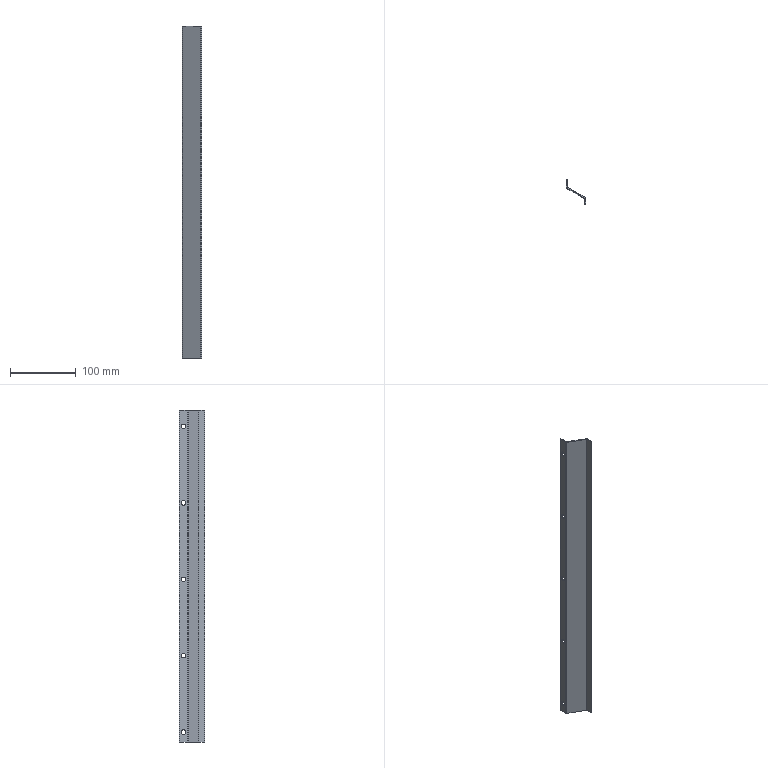Part | STEP file | Right Small Door Splash Plate | 1 solid | 24 faces | box 29.5 x 38.166 x 504 mm | volume 40648 mm3 | cylinder 14 | plane 10 | commonest cylinder face diameters 7 x10 0.2 x2 3.2 x2
STEP:
#1=CARTESIAN_POINT('',(-46.603,-10.206,479.));
#2=VERTEX_POINT('',#1);
#3=CARTESIAN_POINT('',(-46.603,-3.206,479.));
#4=VERTEX_POINT('',#3);
#5=CARTESIAN_POINT('',(-46.603,-6.706,479.));
#6=DIRECTION('',(1.,0.,0.));
#7=DIRECTION('',(0.,1.,0.));
#8=AXIS2_PLACEMENT_3D('',#5,#6,#7);
#9=CIRCLE('',#8,3.5);
#10=EDGE_CURVE('',#2,#4,#9,.T.);
#11=ORIENTED_EDGE('',*,*,#10,.F.);
#12=CARTESIAN_POINT('',(-45.103,-10.206,479.));
#13=VERTEX_POINT('',#12);
#14=CARTESIAN_POINT('',(-55.103,-10.206,479.));
#15=DIRECTION('',(1.,0.,0.));
#16=VECTOR('',#15,1000.);
#17=LINE('',#14,#16);
#18=EDGE_CURVE('',#2,#13,#17,.T.);
#19=ORIENTED_EDGE('',*,*,#18,.T.);
#20=CARTESIAN_POINT('',(-45.103,-3.206,479.));
#21=VERTEX_POINT('',#20);
#22=CARTESIAN_POINT('',(-45.103,-6.706,479.));
#23=DIRECTION('',(-1.,0.,0.));
#24=DIRECTION('',(0.,1.,0.));
#25=AXIS2_PLACEMENT_3D('',#22,#23,#24);
#26=CIRCLE('',#25,3.5);
#27=EDGE_CURVE('',#21,#13,#26,.T.);
#28=ORIENTED_EDGE('',*,*,#27,.F.);
#29=CARTESIAN_POINT('',(-55.103,-3.206,479.));
#30=DIRECTION('',(1.,0.,0.));
#31=VECTOR('',#30,1000.);
#32=LINE('',#29,#31);
#33=EDGE_CURVE('',#4,#21,#32,.T.);
#34=ORIENTED_EDGE('',*,*,#33,.F.);
#35=EDGE_LOOP('',(#11,#19,#28,#34));
#36=FACE_OUTER_BOUND('',#35,.T.);
#37=CARTESIAN_POINT('',(-55.103,-6.706,479.));
#38=DIRECTION('',(1.,0.,0.));
#39=DIRECTION('',(0.,1.,0.));
#40=AXIS2_PLACEMENT_3D('',#37,#38,#39);
#41=CYLINDRICAL_SURFACE('',#40,3.5);
#42=ADVANCED_FACE('',(#36),#41,.F.);
#43=CARTESIAN_POINT('',(-46.603,-10.206,363.));
#44=VERTEX_POINT('',#43);
#45=CARTESIAN_POINT('',(-46.603,-3.206,363.));
#46=VERTEX_POINT('',#45);
#47=CARTESIAN_POINT('',(-46.603,-6.706,363.));
#48=DIRECTION('',(1.,0.,0.));
#49=DIRECTION('',(0.,1.,0.));
#50=AXIS2_PLACEMENT_3D('',#47,#48,#49);
#51=CIRCLE('',#50,3.5);
#52=EDGE_CURVE('',#44,#46,#51,.T.);
#53=ORIENTED_EDGE('',*,*,#52,.F.);
#54=CARTESIAN_POINT('',(-45.103,-10.206,363.));
#55=VERTEX_POINT('',#54);
#56=CARTESIAN_POINT('',(-55.103,-10.206,363.));
#57=DIRECTION('',(1.,0.,0.));
#58=VECTOR('',#57,1000.);
#59=LINE('',#56,#58);
#60=EDGE_CURVE('',#44,#55,#59,.T.);
#61=ORIENTED_EDGE('',*,*,#60,.T.);
#62=CARTESIAN_POINT('',(-45.103,-3.206,363.));
#63=VERTEX_POINT('',#62);
#64=CARTESIAN_POINT('',(-45.103,-6.706,363.));
#65=DIRECTION('',(-1.,0.,0.));
#66=DIRECTION('',(0.,1.,0.));
#67=AXIS2_PLACEMENT_3D('',#64,#65,#66);
#68=CIRCLE('',#67,3.5);
#69=EDGE_CURVE('',#63,#55,#68,.T.);
#70=ORIENTED_EDGE('',*,*,#69,.F.);
#71=CARTESIAN_POINT('',(-55.103,-3.206,363.));
#72=DIRECTION('',(1.,0.,0.));
#73=VECTOR('',#72,1000.);
#74=LINE('',#71,#73);
#75=EDGE_CURVE('',#46,#63,#74,.T.);
#76=ORIENTED_EDGE('',*,*,#75,.F.);
#77=EDGE_LOOP('',(#53,#61,#70,#76));
#78=FACE_OUTER_BOUND('',#77,.T.);
#79=CARTESIAN_POINT('',(-55.103,-6.706,363.));
#80=DIRECTION('',(1.,0.,0.));
#81=DIRECTION('',(0.,1.,0.));
#82=AXIS2_PLACEMENT_3D('',#79,#80,#81);
#83=CYLINDRICAL_SURFACE('',#82,3.5);
#84=ADVANCED_FACE('',(#78),#83,.F.);
#85=CARTESIAN_POINT('',(-46.603,-10.206,247.));
#86=VERTEX_POINT('',#85);
#87=CARTESIAN_POINT('',(-46.603,-3.206,247.));
#88=VERTEX_POINT('',#87);
#89=CARTESIAN_POINT('',(-46.603,-6.706,247.));
#90=DIRECTION('',(1.,0.,0.));
#91=DIRECTION('',(0.,1.,0.));
#92=AXIS2_PLACEMENT_3D('',#89,#90,#91);
#93=CIRCLE('',#92,3.5);
#94=EDGE_CURVE('',#86,#88,#93,.T.);
#95=ORIENTED_EDGE('',*,*,#94,.F.);
#96=CARTESIAN_POINT('',(-45.103,-10.206,247.));
#97=VERTEX_POINT('',#96);
#98=CARTESIAN_POINT('',(-55.103,-10.206,247.));
#99=DIRECTION('',(1.,0.,0.));
#100=VECTOR('',#99,1000.);
#101=LINE('',#98,#100);
#102=EDGE_CURVE('',#86,#97,#101,.T.);
#103=ORIENTED_EDGE('',*,*,#102,.T.);
#104=CARTESIAN_POINT('',(-45.103,-3.206,247.));
#105=VERTEX_POINT('',#104);
#106=CARTESIAN_POINT('',(-45.103,-6.706,247.));
#107=DIRECTION('',(-1.,0.,0.));
#108=DIRECTION('',(0.,1.,0.));
#109=AXIS2_PLACEMENT_3D('',#106,#107,#108);
#110=CIRCLE('',#109,3.5);
#111=EDGE_CURVE('',#105,#97,#110,.T.);
#112=ORIENTED_EDGE('',*,*,#111,.F.);
#113=CARTESIAN_POINT('',(-55.103,-3.206,247.));
#114=DIRECTION('',(1.,0.,0.));
#115=VECTOR('',#114,1000.);
#116=LINE('',#113,#115);
#117=EDGE_CURVE('',#88,#105,#116,.T.);
#118=ORIENTED_EDGE('',*,*,#117,.F.);
#119=EDGE_LOOP('',(#95,#103,#112,#118));
#120=FACE_OUTER_BOUND('',#119,.T.);
#121=CARTESIAN_POINT('',(-55.103,-6.706,247.));
#122=DIRECTION('',(1.,0.,0.));
#123=DIRECTION('',(0.,1.,0.));
#124=AXIS2_PLACEMENT_3D('',#121,#122,#123);
#125=CYLINDRICAL_SURFACE('',#124,3.5);
#126=ADVANCED_FACE('',(#120),#125,.F.);
#127=CARTESIAN_POINT('',(-46.603,-10.206,131.));
#128=VERTEX_POINT('',#127);
#129=CARTESIAN_POINT('',(-46.603,-3.206,131.));
#130=VERTEX_POINT('',#129);
#131=CARTESIAN_POINT('',(-46.603,-6.706,131.));
#132=DIRECTION('',(1.,0.,0.));
#133=DIRECTION('',(0.,1.,0.));
#134=AXIS2_PLACEMENT_3D('',#131,#132,#133);
#135=CIRCLE('',#134,3.5);
#136=EDGE_CURVE('',#128,#130,#135,.T.);
#137=ORIENTED_EDGE('',*,*,#136,.F.);
#138=CARTESIAN_POINT('',(-45.103,-10.206,131.));
#139=VERTEX_POINT('',#138);
#140=CARTESIAN_POINT('',(-55.103,-10.206,131.));
#141=DIRECTION('',(1.,0.,0.));
#142=VECTOR('',#141,1000.);
#143=LINE('',#140,#142);
#144=EDGE_CURVE('',#128,#139,#143,.T.);
#145=ORIENTED_EDGE('',*,*,#144,.T.);
#146=CARTESIAN_POINT('',(-45.103,-3.206,131.));
#147=VERTEX_POINT('',#146);
#148=CARTESIAN_POINT('',(-45.103,-6.706,131.));
#149=DIRECTION('',(-1.,0.,0.));
#150=DIRECTION('',(0.,1.,0.));
#151=AXIS2_PLACEMENT_3D('',#148,#149,#150);
#152=CIRCLE('',#151,3.5);
#153=EDGE_CURVE('',#147,#139,#152,.T.);
#154=ORIENTED_EDGE('',*,*,#153,.F.);
#155=CARTESIAN_POINT('',(-55.103,-3.206,131.));
#156=DIRECTION('',(1.,0.,0.));
#157=VECTOR('',#156,1000.);
#158=LINE('',#155,#157);
#159=EDGE_CURVE('',#130,#147,#158,.T.);
#160=ORIENTED_EDGE('',*,*,#159,.F.);
#161=EDGE_LOOP('',(#137,#145,#154,#160));
#162=FACE_OUTER_BOUND('',#161,.T.);
#163=CARTESIAN_POINT('',(-55.103,-6.706,131.));
#164=DIRECTION('',(1.,0.,0.));
#165=DIRECTION('',(0.,1.,0.));
#166=AXIS2_PLACEMENT_3D('',#163,#164,#165);
#167=CYLINDRICAL_SURFACE('',#166,3.5);
#168=ADVANCED_FACE('',(#162),#167,.F.);
#169=CARTESIAN_POINT('',(-46.603,-10.206,15.));
#170=VERTEX_POINT('',#169);
#171=CARTESIAN_POINT('',(-46.603,-3.206,15.));
#172=VERTEX_POINT('',#171);
#173=CARTESIAN_POINT('',(-46.603,-6.706,15.));
#174=DIRECTION('',(1.,0.,0.));
#175=DIRECTION('',(0.,1.,0.));
#176=AXIS2_PLACEMENT_3D('',#173,#174,#175);
#177=CIRCLE('',#176,3.5);
#178=EDGE_CURVE('',#170,#172,#177,.T.);
#179=ORIENTED_EDGE('',*,*,#178,.F.);
#180=CARTESIAN_POINT('',(-45.103,-10.206,15.));
#181=VERTEX_POINT('',#180);
#182=CARTESIAN_POINT('',(-55.103,-10.206,15.));
#183=DIRECTION('',(1.,0.,0.));
#184=VECTOR('',#183,1000.);
#185=LINE('',#182,#184);
#186=EDGE_CURVE('',#170,#181,#185,.T.);
#187=ORIENTED_EDGE('',*,*,#186,.T.);
#188=CARTESIAN_POINT('',(-45.103,-3.206,15.));
#189=VERTEX_POINT('',#188);
#190=CARTESIAN_POINT('',(-45.103,-6.706,15.));
#191=DIRECTION('',(-1.,0.,0.));
#192=DIRECTION('',(0.,1.,0.));
#193=AXIS2_PLACEMENT_3D('',#190,#191,#192);
#194=CIRCLE('',#193,3.5);
#195=EDGE_CURVE('',#189,#181,#194,.T.);
#196=ORIENTED_EDGE('',*,*,#195,.F.);
#197=CARTESIAN_POINT('',(-55.103,-3.206,15.));
#198=DIRECTION('',(1.,0.,0.));
#199=VECTOR('',#198,1000.);
#200=LINE('',#197,#199);
#201=EDGE_CURVE('',#172,#189,#200,.T.);
#202=ORIENTED_EDGE('',*,*,#201,.F.);
#203=EDGE_LOOP('',(#179,#187,#196,#202));
#204=FACE_OUTER_BOUND('',#203,.T.);
#205=CARTESIAN_POINT('',(-55.103,-6.706,15.));
#206=DIRECTION('',(1.,0.,0.));
#207=DIRECTION('',(0.,1.,0.));
#208=AXIS2_PLACEMENT_3D('',#205,#206,#207);
#209=CYLINDRICAL_SURFACE('',#208,3.5);
#210=ADVANCED_FACE('',(#204),#209,.F.);
#211=CARTESIAN_POINT('',(-45.053,-12.764,504.));
#212=VERTEX_POINT('',#211);
#213=CARTESIAN_POINT('',(-17.903,-28.439,504.));
#214=VERTEX_POINT('',#213);
#215=CARTESIAN_POINT('',(-45.103,-12.735,504.));
#216=DIRECTION('',(0.866,-0.5,0.));
#217=VECTOR('',#216,1000.);
#218=LINE('',#215,#217);
#219=EDGE_CURVE('',#212,#214,#218,.T.);
#220=ORIENTED_EDGE('',*,*,#219,.T.);
#221=CARTESIAN_POINT('',(-17.903,-28.439,0.));
#222=VERTEX_POINT('',#221);
#223=CARTESIAN_POINT('',(-17.903,-28.439,504.));
#224=DIRECTION('',(0.,0.,-1.));
#225=VECTOR('',#224,1000.);
#226=LINE('',#223,#225);
#227=EDGE_CURVE('',#214,#222,#226,.T.);
#228=ORIENTED_EDGE('',*,*,#227,.T.);
#229=CARTESIAN_POINT('',(-45.053,-12.764,0.));
#230=VERTEX_POINT('',#229);
#231=CARTESIAN_POINT('',(-45.103,-12.735,0.));
#232=DIRECTION('',(-0.866,0.5,0.));
#233=VECTOR('',#232,1000.);
#234=LINE('',#231,#233);
#235=EDGE_CURVE('',#222,#230,#234,.T.);
#236=ORIENTED_EDGE('',*,*,#235,.T.);
#237=CARTESIAN_POINT('',(-45.053,-12.764,504.));
#238=DIRECTION('',(0.,0.,1.));
#239=VECTOR('',#238,1000.);
#240=LINE('',#237,#239);
#241=EDGE_CURVE('',#230,#212,#240,.T.);
#242=ORIENTED_EDGE('',*,*,#241,.T.);
#243=EDGE_LOOP('',(#220,#228,#236,#242));
#244=FACE_OUTER_BOUND('',#243,.T.);
#245=CARTESIAN_POINT('',(-45.103,-12.735,504.));
#246=DIRECTION('',(0.5,0.866,0.));
#247=DIRECTION('',(-0.866,0.5,0.));
#248=AXIS2_PLACEMENT_3D('',#245,#246,#247);
#249=PLANE('',#248);
#250=ADVANCED_FACE('',(#244),#249,.T.);
#251=CARTESIAN_POINT('',(-17.103,-29.824,504.));
#252=VERTEX_POINT('',#251);
#253=CARTESIAN_POINT('',(-18.703,-29.824,504.));
#254=DIRECTION('',(0.,0.,-1.));
#255=DIRECTION('',(-1.,0.,0.));
#256=AXIS2_PLACEMENT_3D('',#253,#254,#255);
#257=CIRCLE('',#256,1.6);
#258=EDGE_CURVE('',#214,#252,#257,.T.);
#259=ORIENTED_EDGE('',*,*,#258,.T.);
#260=CARTESIAN_POINT('',(-17.103,-29.824,0.));
#261=VERTEX_POINT('',#260);
#262=CARTESIAN_POINT('',(-17.103,-29.824,504.));
#263=DIRECTION('',(0.,0.,-1.));
#264=VECTOR('',#263,1000.);
#265=LINE('',#262,#264);
#266=EDGE_CURVE('',#252,#261,#265,.T.);
#267=ORIENTED_EDGE('',*,*,#266,.T.);
#268=CARTESIAN_POINT('',(-18.703,-29.824,0.));
#269=DIRECTION('',(0.,0.,1.));
#270=DIRECTION('',(-1.,0.,0.));
#271=AXIS2_PLACEMENT_3D('',#268,#269,#270);
#272=CIRCLE('',#271,1.6);
#273=EDGE_CURVE('',#261,#222,#272,.T.);
#274=ORIENTED_EDGE('',*,*,#273,.T.);
#275=ORIENTED_EDGE('',*,*,#227,.F.);
#276=EDGE_LOOP('',(#259,#267,#274,#275));
#277=FACE_OUTER_BOUND('',#276,.T.);
#278=CARTESIAN_POINT('',(-18.703,-29.824,504.));
#279=DIRECTION('',(0.,0.,-1.));
#280=DIRECTION('',(-1.,0.,0.));
#281=AXIS2_PLACEMENT_3D('',#278,#279,#280);
#282=CYLINDRICAL_SURFACE('',#281,1.6);
#283=ADVANCED_FACE('',(#277),#282,.T.);
#284=CARTESIAN_POINT('',(-45.803,-14.063,504.));
#285=VERTEX_POINT('',#284);
#286=CARTESIAN_POINT('',(-18.653,-29.738,504.));
#287=VERTEX_POINT('',#286);
#288=CARTESIAN_POINT('',(-45.803,-14.063,504.));
#289=DIRECTION('',(0.866,-0.5,0.));
#290=VECTOR('',#289,1000.);
#291=LINE('',#288,#290);
#292=EDGE_CURVE('',#285,#287,#291,.T.);
#293=ORIENTED_EDGE('',*,*,#292,.T.);
#294=CARTESIAN_POINT('',(-18.603,-29.824,504.));
#295=VERTEX_POINT('',#294);
#296=CARTESIAN_POINT('',(-18.703,-29.824,504.));
#297=DIRECTION('',(0.,0.,-1.));
#298=DIRECTION('',(-1.,0.,0.));
#299=AXIS2_PLACEMENT_3D('',#296,#297,#298);
#300=CIRCLE('',#299,0.1);
#301=EDGE_CURVE('',#287,#295,#300,.T.);
#302=ORIENTED_EDGE('',*,*,#301,.T.);
#303=CARTESIAN_POINT('',(-18.603,-38.901,504.));
#304=VERTEX_POINT('',#303);
#305=CARTESIAN_POINT('',(-18.603,-29.738,504.));
#306=DIRECTION('',(0.,-1.,0.));
#307=VECTOR('',#306,1000.);
#308=LINE('',#305,#307);
#309=EDGE_CURVE('',#295,#304,#308,.T.);
#310=ORIENTED_EDGE('',*,*,#309,.T.);
#311=CARTESIAN_POINT('',(-17.103,-38.901,504.));
#312=VERTEX_POINT('',#311);
#313=CARTESIAN_POINT('',(-17.103,-38.901,504.));
#314=DIRECTION('',(-1.,0.,0.));
#315=VECTOR('',#314,1000.);
#316=LINE('',#313,#315);
#317=EDGE_CURVE('',#312,#304,#316,.T.);
#318=ORIENTED_EDGE('',*,*,#317,.F.);
#319=CARTESIAN_POINT('',(-17.103,-28.901,504.));
#320=DIRECTION('',(0.,-1.,0.));
#321=VECTOR('',#320,1000.);
#322=LINE('',#319,#321);
#323=EDGE_CURVE('',#252,#312,#322,.T.);
#324=ORIENTED_EDGE('',*,*,#323,.F.);
#325=ORIENTED_EDGE('',*,*,#258,.F.);
#326=ORIENTED_EDGE('',*,*,#219,.F.);
#327=CARTESIAN_POINT('',(-45.103,-12.677,504.));
#328=VERTEX_POINT('',#327);
#329=CARTESIAN_POINT('',(-45.003,-12.677,504.));
#330=DIRECTION('',(0.,0.,-1.));
#331=DIRECTION('',(-1.,0.,0.));
#332=AXIS2_PLACEMENT_3D('',#329,#330,#331);
#333=CIRCLE('',#332,0.1);
#334=EDGE_CURVE('',#212,#328,#333,.T.);
#335=ORIENTED_EDGE('',*,*,#334,.T.);
#336=CARTESIAN_POINT('',(-45.103,-0.7348,504.));
#337=VERTEX_POINT('',#336);
#338=CARTESIAN_POINT('',(-45.103,-0.7348,504.));
#339=DIRECTION('',(0.,-1.,0.));
#340=VECTOR('',#339,1000.);
#341=LINE('',#338,#340);
#342=EDGE_CURVE('',#337,#328,#341,.T.);
#343=ORIENTED_EDGE('',*,*,#342,.F.);
#344=CARTESIAN_POINT('',(-46.603,-0.7348,504.));
#345=VERTEX_POINT('',#344);
#346=CARTESIAN_POINT('',(-18.703,-0.7348,504.));
#347=DIRECTION('',(-1.,0.,0.));
#348=VECTOR('',#347,1000.);
#349=LINE('',#346,#348);
#350=EDGE_CURVE('',#337,#345,#349,.T.);
#351=ORIENTED_EDGE('',*,*,#350,.T.);
#352=CARTESIAN_POINT('',(-46.603,-12.677,504.));
#353=VERTEX_POINT('',#352);
#354=CARTESIAN_POINT('',(-46.603,-29.824,504.));
#355=DIRECTION('',(0.,-1.,0.));
#356=VECTOR('',#355,1000.);
#357=LINE('',#354,#356);
#358=EDGE_CURVE('',#345,#353,#357,.T.);
#359=ORIENTED_EDGE('',*,*,#358,.T.);
#360=CARTESIAN_POINT('',(-45.003,-12.677,504.));
#361=DIRECTION('',(0.,0.,1.));
#362=DIRECTION('',(-1.,0.,0.));
#363=AXIS2_PLACEMENT_3D('',#360,#361,#362);
#364=CIRCLE('',#363,1.6);
#365=EDGE_CURVE('',#353,#285,#364,.T.);
#366=ORIENTED_EDGE('',*,*,#365,.T.);
#367=EDGE_LOOP('',(#293,#302,#310,#318,#324,#325,#326,#335,#343,#351,#359,#366));
#368=FACE_OUTER_BOUND('',#367,.T.);
#369=CARTESIAN_POINT('',(-46.603,-12.677,504.));
#370=DIRECTION('',(0.,0.,1.));
#371=DIRECTION('',(1.,0.,0.));
#372=AXIS2_PLACEMENT_3D('',#369,#370,#371);
#373=PLANE('',#372);
#374=ADVANCED_FACE('',(#368),#373,.T.);
#375=CARTESIAN_POINT('',(-45.103,-12.677,0.));
#376=VERTEX_POINT('',#375);
#377=CARTESIAN_POINT('',(-45.103,-12.677,504.));
#378=DIRECTION('',(0.,0.,-1.));
#379=VECTOR('',#378,1000.);
#380=LINE('',#377,#379);
#381=EDGE_CURVE('',#328,#376,#380,.T.);
#382=ORIENTED_EDGE('',*,*,#381,.F.);
#383=ORIENTED_EDGE('',*,*,#334,.F.);
#384=ORIENTED_EDGE('',*,*,#241,.F.);
#385=CARTESIAN_POINT('',(-45.003,-12.677,0.));
#386=DIRECTION('',(0.,0.,1.));
#387=DIRECTION('',(-1.,0.,0.));
#388=AXIS2_PLACEMENT_3D('',#385,#386,#387);
#389=CIRCLE('',#388,0.1);
#390=EDGE_CURVE('',#376,#230,#389,.T.);
#391=ORIENTED_EDGE('',*,*,#390,.F.);
#392=EDGE_LOOP('',(#382,#383,#384,#391));
#393=FACE_OUTER_BOUND('',#392,.T.);
#394=CARTESIAN_POINT('',(-45.003,-12.677,504.));
#395=DIRECTION('',(0.,0.,-1.));
#396=DIRECTION('',(-1.,0.,0.));
#397=AXIS2_PLACEMENT_3D('',#394,#395,#396);
#398=CYLINDRICAL_SURFACE('',#397,0.1);
#399=ADVANCED_FACE('',(#393),#398,.F.);
#400=CARTESIAN_POINT('',(-18.653,-29.738,0.));
#401=VERTEX_POINT('',#400);
#402=CARTESIAN_POINT('',(-45.803,-14.063,0.));
#403=VERTEX_POINT('',#402);
#404=CARTESIAN_POINT('',(-18.653,-29.738,0.));
#405=DIRECTION('',(-0.866,0.5,0.));
#406=VECTOR('',#405,1000.);
#407=LINE('',#404,#406);
#408=EDGE_CURVE('',#401,#403,#407,.T.);
#409=ORIENTED_EDGE('',*,*,#408,.T.);
#410=CARTESIAN_POINT('',(-46.603,-12.677,0.));
#411=VERTEX_POINT('',#410);
#412=CARTESIAN_POINT('',(-45.003,-12.677,0.));
#413=DIRECTION('',(0.,0.,-1.));
#414=DIRECTION('',(-1.,0.,0.));
#415=AXIS2_PLACEMENT_3D('',#412,#413,#414);
#416=CIRCLE('',#415,1.6);
#417=EDGE_CURVE('',#403,#411,#416,.T.);
#418=ORIENTED_EDGE('',*,*,#417,.T.);
#419=CARTESIAN_POINT('',(-46.603,-0.7348,0.));
#420=VERTEX_POINT('',#419);
#421=CARTESIAN_POINT('',(-46.603,-14.063,0.));
#422=DIRECTION('',(0.,1.,0.));
#423=VECTOR('',#422,1000.);
#424=LINE('',#421,#423);
#425=EDGE_CURVE('',#411,#420,#424,.T.);
#426=ORIENTED_EDGE('',*,*,#425,.T.);
#427=CARTESIAN_POINT('',(-45.103,-0.7348,0.));
#428=VERTEX_POINT('',#427);
#429=CARTESIAN_POINT('',(-46.603,-0.7348,0.));
#430=DIRECTION('',(-1.,0.,0.));
#431=VECTOR('',#430,1000.);
#432=LINE('',#429,#431);
#433=EDGE_CURVE('',#428,#420,#432,.T.);
#434=ORIENTED_EDGE('',*,*,#433,.F.);
#435=CARTESIAN_POINT('',(-45.103,-0.7348,0.));
#436=DIRECTION('',(0.,1.,0.));
#437=VECTOR('',#436,1000.);
#438=LINE('',#435,#437);
#439=EDGE_CURVE('',#376,#428,#438,.T.);
#440=ORIENTED_EDGE('',*,*,#439,.F.);
#441=ORIENTED_EDGE('',*,*,#390,.T.);
#442=ORIENTED_EDGE('',*,*,#235,.F.);
#443=ORIENTED_EDGE('',*,*,#273,.F.);
#444=CARTESIAN_POINT('',(-17.103,-38.901,0.));
#445=VERTEX_POINT('',#444);
#446=CARTESIAN_POINT('',(-17.103,-28.901,0.));
#447=DIRECTION('',(0.,1.,0.));
#448=VECTOR('',#447,1000.);
#449=LINE('',#446,#448);
#450=EDGE_CURVE('',#445,#261,#449,.T.);
#451=ORIENTED_EDGE('',*,*,#450,.F.);
#452=CARTESIAN_POINT('',(-18.603,-38.901,0.));
#453=VERTEX_POINT('',#452);
#454=CARTESIAN_POINT('',(-17.103,-38.901,0.));
#455=DIRECTION('',(1.,0.,0.));
#456=VECTOR('',#455,1000.);
#457=LINE('',#454,#456);
#458=EDGE_CURVE('',#453,#445,#457,.T.);
#459=ORIENTED_EDGE('',*,*,#458,.F.);
#460=CARTESIAN_POINT('',(-18.603,-29.824,0.));
#461=VERTEX_POINT('',#460);
#462=CARTESIAN_POINT('',(-18.603,-29.824,0.));
#463=DIRECTION('',(0.,-1.,0.));
#464=VECTOR('',#463,1000.);
#465=LINE('',#462,#464);
#466=EDGE_CURVE('',#461,#453,#465,.T.);
#467=ORIENTED_EDGE('',*,*,#466,.F.);
#468=CARTESIAN_POINT('',(-18.703,-29.824,0.));
#469=DIRECTION('',(0.,0.,1.));
#470=DIRECTION('',(-1.,0.,0.));
#471=AXIS2_PLACEMENT_3D('',#468,#469,#470);
#472=CIRCLE('',#471,0.1);
#473=EDGE_CURVE('',#461,#401,#472,.T.);
#474=ORIENTED_EDGE('',*,*,#473,.T.);
#475=EDGE_LOOP('',(#409,#418,#426,#434,#440,#441,#442,#443,#451,#459,#467,#474));
#476=FACE_OUTER_BOUND('',#475,.T.);
#477=CARTESIAN_POINT('',(-18.603,-29.824,0.));
#478=DIRECTION('',(0.,0.,-1.));
#479=DIRECTION('',(-1.,0.,0.));
#480=AXIS2_PLACEMENT_3D('',#477,#478,#479);
#481=PLANE('',#480);
#482=ADVANCED_FACE('',(#476),#481,.T.);
#483=ORIENTED_EDGE('',*,*,#323,.T.);
#484=CARTESIAN_POINT('',(-17.103,-38.901,504.));
#485=DIRECTION('',(0.,0.,-1.));
#486=VECTOR('',#485,1000.);
#487=LINE('',#484,#486);
#488=EDGE_CURVE('',#312,#445,#487,.T.);
#489=ORIENTED_EDGE('',*,*,#488,.T.);
#490=ORIENTED_EDGE('',*,*,#450,.T.);
#491=ORIENTED_EDGE('',*,*,#266,.F.);
#492=EDGE_LOOP('',(#483,#489,#490,#491));
#493=FACE_OUTER_BOUND('',#492,.T.);
#494=CARTESIAN_POINT('',(-17.103,-28.901,504.));
#495=DIRECTION('',(1.,0.,0.));
#496=DIRECTION('',(0.,1.,0.));
#497=AXIS2_PLACEMENT_3D('',#494,#495,#496);
#498=PLANE('',#497);
#499=ADVANCED_FACE('',(#493),#498,.T.);
#500=CARTESIAN_POINT('',(-18.653,-29.738,504.));
#501=DIRECTION('',(0.,0.,-1.));
#502=VECTOR('',#501,1000.);
#503=LINE('',#500,#502);
#504=EDGE_CURVE('',#287,#401,#503,.T.);
#505=ORIENTED_EDGE('',*,*,#504,.F.);
#506=ORIENTED_EDGE('',*,*,#292,.F.);
#507=CARTESIAN_POINT('',(-45.803,-14.063,504.));
#508=DIRECTION('',(0.,0.,1.));
#509=VECTOR('',#508,1000.);
#510=LINE('',#507,#509);
#511=EDGE_CURVE('',#403,#285,#510,.T.);
#512=ORIENTED_EDGE('',*,*,#511,.F.);
#513=ORIENTED_EDGE('',*,*,#408,.F.);
#514=EDGE_LOOP('',(#505,#506,#512,#513));
#515=FACE_OUTER_BOUND('',#514,.T.);
#516=CARTESIAN_POINT('',(-45.853,-14.034,504.));
#517=DIRECTION('',(0.5,0.866,0.));
#518=DIRECTION('',(-0.866,0.5,0.));
#519=AXIS2_PLACEMENT_3D('',#516,#517,#518);
#520=PLANE('',#519);
#521=ADVANCED_FACE('',(#515),#520,.F.);
#522=ORIENTED_EDGE('',*,*,#342,.T.);
#523=ORIENTED_EDGE('',*,*,#381,.T.);
#524=ORIENTED_EDGE('',*,*,#439,.T.);
#525=CARTESIAN_POINT('',(-45.103,-0.7348,504.));
#526=DIRECTION('',(0.,0.,1.));
#527=VECTOR('',#526,1000.);
#528=LINE('',#525,#527);
#529=EDGE_CURVE('',#428,#337,#528,.T.);
#530=ORIENTED_EDGE('',*,*,#529,.T.);
#531=EDGE_LOOP('',(#522,#523,#524,#530));
#532=FACE_OUTER_BOUND('',#531,.T.);
#533=ORIENTED_EDGE('',*,*,#27,.T.);
#534=CARTESIAN_POINT('',(-45.103,-6.706,479.));
#535=DIRECTION('',(-1.,0.,0.));
#536=DIRECTION('',(0.,1.,0.));
#537=AXIS2_PLACEMENT_3D('',#534,#535,#536);
#538=CIRCLE('',#537,3.5);
#539=EDGE_CURVE('',#13,#21,#538,.T.);
#540=ORIENTED_EDGE('',*,*,#539,.T.);
#541=EDGE_LOOP('',(#533,#540));
#542=FACE_BOUND('',#541,.T.);
#543=ORIENTED_EDGE('',*,*,#69,.T.);
#544=CARTESIAN_POINT('',(-45.103,-6.706,363.));
#545=DIRECTION('',(-1.,0.,0.));
#546=DIRECTION('',(0.,1.,0.));
#547=AXIS2_PLACEMENT_3D('',#544,#545,#546);
#548=CIRCLE('',#547,3.5);
#549=EDGE_CURVE('',#55,#63,#548,.T.);
#550=ORIENTED_EDGE('',*,*,#549,.T.);
#551=EDGE_LOOP('',(#543,#550));
#552=FACE_BOUND('',#551,.T.);
#553=ORIENTED_EDGE('',*,*,#111,.T.);
#554=CARTESIAN_POINT('',(-45.103,-6.706,247.));
#555=DIRECTION('',(-1.,0.,0.));
#556=DIRECTION('',(0.,1.,0.));
#557=AXIS2_PLACEMENT_3D('',#554,#555,#556);
#558=CIRCLE('',#557,3.5);
#559=EDGE_CURVE('',#97,#105,#558,.T.);
#560=ORIENTED_EDGE('',*,*,#559,.T.);
#561=EDGE_LOOP('',(#553,#560));
#562=FACE_BOUND('',#561,.T.);
#563=ORIENTED_EDGE('',*,*,#153,.T.);
#564=CARTESIAN_POINT('',(-45.103,-6.706,131.));
#565=DIRECTION('',(-1.,0.,0.));
#566=DIRECTION('',(0.,1.,0.));
#567=AXIS2_PLACEMENT_3D('',#564,#565,#566);
#568=CIRCLE('',#567,3.5);
#569=EDGE_CURVE('',#139,#147,#568,.T.);
#570=ORIENTED_EDGE('',*,*,#569,.T.);
#571=EDGE_LOOP('',(#563,#570));
#572=FACE_BOUND('',#571,.T.);
#573=ORIENTED_EDGE('',*,*,#195,.T.);
#574=CARTESIAN_POINT('',(-45.103,-6.706,15.));
#575=DIRECTION('',(-1.,0.,0.));
#576=DIRECTION('',(0.,1.,0.));
#577=AXIS2_PLACEMENT_3D('',#574,#575,#576);
#578=CIRCLE('',#577,3.5);
#579=EDGE_CURVE('',#181,#189,#578,.T.);
#580=ORIENTED_EDGE('',*,*,#579,.T.);
#581=EDGE_LOOP('',(#573,#580));
#582=FACE_BOUND('',#581,.T.);
#583=CARTESIAN_POINT('',(-45.103,-0.7348,504.));
#584=DIRECTION('',(1.,0.,0.));
#585=DIRECTION('',(0.,1.,0.));
#586=AXIS2_PLACEMENT_3D('',#583,#584,#585);
#587=PLANE('',#586);
#588=ADVANCED_FACE('',(#532,#542,#552,#562,#572,#582),#587,.T.);
#589=ORIENTED_EDGE('',*,*,#317,.T.);
#590=CARTESIAN_POINT('',(-18.603,-38.901,504.));
#591=DIRECTION('',(0.,0.,-1.));
#592=VECTOR('',#591,1000.);
#593=LINE('',#590,#592);
#594=EDGE_CURVE('',#304,#453,#593,.T.);
#595=ORIENTED_EDGE('',*,*,#594,.T.);
#596=ORIENTED_EDGE('',*,*,#458,.T.);
#597=ORIENTED_EDGE('',*,*,#488,.F.);
#598=EDGE_LOOP('',(#589,#595,#596,#597));
#599=FACE_OUTER_BOUND('',#598,.T.);
#600=CARTESIAN_POINT('',(-17.103,-38.901,504.));
#601=DIRECTION('',(0.,-1.,0.));
#602=DIRECTION('',(0.,0.,-1.));
#603=AXIS2_PLACEMENT_3D('',#600,#601,#602);
#604=PLANE('',#603);
#605=ADVANCED_FACE('',(#599),#604,.T.);
#606=CARTESIAN_POINT('',(-18.603,-29.824,504.));
#607=DIRECTION('',(0.,0.,-1.));
#608=VECTOR('',#607,1000.);
#609=LINE('',#606,#608);
#610=EDGE_CURVE('',#295,#461,#609,.T.);
#611=ORIENTED_EDGE('',*,*,#610,.F.);
#612=ORIENTED_EDGE('',*,*,#301,.F.);
#613=ORIENTED_EDGE('',*,*,#504,.T.);
#614=ORIENTED_EDGE('',*,*,#473,.F.);
#615=EDGE_LOOP('',(#611,#612,#613,#614));
#616=FACE_OUTER_BOUND('',#615,.T.);
#617=CARTESIAN_POINT('',(-18.703,-29.824,504.));
#618=DIRECTION('',(0.,0.,-1.));
#619=DIRECTION('',(-1.,0.,0.));
#620=AXIS2_PLACEMENT_3D('',#617,#618,#619);
#621=CYLINDRICAL_SURFACE('',#620,0.1);
#622=ADVANCED_FACE('',(#616),#621,.F.);
#623=ORIENTED_EDGE('',*,*,#365,.F.);
#624=CARTESIAN_POINT('',(-46.603,-12.677,504.));
#625=DIRECTION('',(0.,0.,-1.));
#626=VECTOR('',#625,1000.);
#627=LINE('',#624,#626);
#628=EDGE_CURVE('',#353,#411,#627,.T.);
#629=ORIENTED_EDGE('',*,*,#628,.T.);
#630=ORIENTED_EDGE('',*,*,#417,.F.);
#631=ORIENTED_EDGE('',*,*,#511,.T.);
#632=EDGE_LOOP('',(#623,#629,#630,#631));
#633=FACE_OUTER_BOUND('',#632,.T.);
#634=CARTESIAN_POINT('',(-45.003,-12.677,504.));
#635=DIRECTION('',(0.,0.,-1.));
#636=DIRECTION('',(-1.,0.,0.));
#637=AXIS2_PLACEMENT_3D('',#634,#635,#636);
#638=CYLINDRICAL_SURFACE('',#637,1.6);
#639=ADVANCED_FACE('',(#633),#638,.T.);
#640=ORIENTED_EDGE('',*,*,#350,.F.);
#641=ORIENTED_EDGE('',*,*,#529,.F.);
#642=ORIENTED_EDGE('',*,*,#433,.T.);
#643=CARTESIAN_POINT('',(-46.603,-0.7348,504.));
#644=DIRECTION('',(0.,0.,1.));
#645=VECTOR('',#644,1000.);
#646=LINE('',#643,#645);
#647=EDGE_CURVE('',#420,#345,#646,.T.);
#648=ORIENTED_EDGE('',*,*,#647,.T.);
#649=EDGE_LOOP('',(#640,#641,#642,#648));
#650=FACE_OUTER_BOUND('',#649,.T.);
#651=CARTESIAN_POINT('',(-46.603,-0.7348,504.));
#652=DIRECTION('',(0.,1.,0.));
#653=DIRECTION('',(-1.,0.,0.));
#654=AXIS2_PLACEMENT_3D('',#651,#652,#653);
#655=PLANE('',#654);
#656=ADVANCED_FACE('',(#650),#655,.T.);
#657=ORIENTED_EDGE('',*,*,#18,.F.);
#658=CARTESIAN_POINT('',(-46.603,-6.706,479.));
#659=DIRECTION('',(1.,0.,0.));
#660=DIRECTION('',(0.,1.,0.));
#661=AXIS2_PLACEMENT_3D('',#658,#659,#660);
#662=CIRCLE('',#661,3.5);
#663=EDGE_CURVE('',#4,#2,#662,.T.);
#664=ORIENTED_EDGE('',*,*,#663,.F.);
#665=ORIENTED_EDGE('',*,*,#33,.T.);
#666=ORIENTED_EDGE('',*,*,#539,.F.);
#667=EDGE_LOOP('',(#657,#664,#665,#666));
#668=FACE_OUTER_BOUND('',#667,.T.);
#669=CARTESIAN_POINT('',(-55.103,-6.706,479.));
#670=DIRECTION('',(1.,0.,0.));
#671=DIRECTION('',(0.,1.,0.));
#672=AXIS2_PLACEMENT_3D('',#669,#670,#671);
#673=CYLINDRICAL_SURFACE('',#672,3.5);
#674=ADVANCED_FACE('',(#668),#673,.F.);
#675=ORIENTED_EDGE('',*,*,#60,.F.);
#676=CARTESIAN_POINT('',(-46.603,-6.706,363.));
#677=DIRECTION('',(1.,0.,0.));
#678=DIRECTION('',(0.,1.,0.));
#679=AXIS2_PLACEMENT_3D('',#676,#677,#678);
#680=CIRCLE('',#679,3.5);
#681=EDGE_CURVE('',#46,#44,#680,.T.);
#682=ORIENTED_EDGE('',*,*,#681,.F.);
#683=ORIENTED_EDGE('',*,*,#75,.T.);
#684=ORIENTED_EDGE('',*,*,#549,.F.);
#685=EDGE_LOOP('',(#675,#682,#683,#684));
#686=FACE_OUTER_BOUND('',#685,.T.);
#687=CARTESIAN_POINT('',(-55.103,-6.706,363.));
#688=DIRECTION('',(1.,0.,0.));
#689=DIRECTION('',(0.,1.,0.));
#690=AXIS2_PLACEMENT_3D('',#687,#688,#689);
#691=CYLINDRICAL_SURFACE('',#690,3.5);
#692=ADVANCED_FACE('',(#686),#691,.F.);
#693=ORIENTED_EDGE('',*,*,#102,.F.);
#694=CARTESIAN_POINT('',(-46.603,-6.706,247.));
#695=DIRECTION('',(1.,0.,0.));
#696=DIRECTION('',(0.,1.,0.));
#697=AXIS2_PLACEMENT_3D('',#694,#695,#696);
#698=CIRCLE('',#697,3.5);
#699=EDGE_CURVE('',#88,#86,#698,.T.);
#700=ORIENTED_EDGE('',*,*,#699,.F.);
#701=ORIENTED_EDGE('',*,*,#117,.T.);
#702=ORIENTED_EDGE('',*,*,#559,.F.);
#703=EDGE_LOOP('',(#693,#700,#701,#702));
#704=FACE_OUTER_BOUND('',#703,.T.);
#705=CARTESIAN_POINT('',(-55.103,-6.706,247.));
#706=DIRECTION('',(1.,0.,0.));
#707=DIRECTION('',(0.,1.,0.));
#708=AXIS2_PLACEMENT_3D('',#705,#706,#707);
#709=CYLINDRICAL_SURFACE('',#708,3.5);
#710=ADVANCED_FACE('',(#704),#709,.F.);
#711=ORIENTED_EDGE('',*,*,#144,.F.);
#712=CARTESIAN_POINT('',(-46.603,-6.706,131.));
#713=DIRECTION('',(1.,0.,0.));
#714=DIRECTION('',(0.,1.,0.));
#715=AXIS2_PLACEMENT_3D('',#712,#713,#714);
#716=CIRCLE('',#715,3.5);
#717=EDGE_CURVE('',#130,#128,#716,.T.);
#718=ORIENTED_EDGE('',*,*,#717,.F.);
#719=ORIENTED_EDGE('',*,*,#159,.T.);
#720=ORIENTED_EDGE('',*,*,#569,.F.);
#721=EDGE_LOOP('',(#711,#718,#719,#720));
#722=FACE_OUTER_BOUND('',#721,.T.);
#723=CARTESIAN_POINT('',(-55.103,-6.706,131.));
#724=DIRECTION('',(1.,0.,0.));
#725=DIRECTION('',(0.,1.,0.));
#726=AXIS2_PLACEMENT_3D('',#723,#724,#725);
#727=CYLINDRICAL_SURFACE('',#726,3.5);
#728=ADVANCED_FACE('',(#722),#727,.F.);
#729=ORIENTED_EDGE('',*,*,#186,.F.);
#730=CARTESIAN_POINT('',(-46.603,-6.706,15.));
#731=DIRECTION('',(1.,0.,0.));
#732=DIRECTION('',(0.,1.,0.));
#733=AXIS2_PLACEMENT_3D('',#730,#731,#732);
#734=CIRCLE('',#733,3.5);
#735=EDGE_CURVE('',#172,#170,#734,.T.);
#736=ORIENTED_EDGE('',*,*,#735,.F.);
#737=ORIENTED_EDGE('',*,*,#201,.T.);
#738=ORIENTED_EDGE('',*,*,#579,.F.);
#739=EDGE_LOOP('',(#729,#736,#737,#738));
#740=FACE_OUTER_BOUND('',#739,.T.);
#741=CARTESIAN_POINT('',(-55.103,-6.706,15.));
#742=DIRECTION('',(1.,0.,0.));
#743=DIRECTION('',(0.,1.,0.));
#744=AXIS2_PLACEMENT_3D('',#741,#742,#743);
#745=CYLINDRICAL_SURFACE('',#744,3.5);
#746=ADVANCED_FACE('',(#740),#745,.F.);
#747=ORIENTED_EDGE('',*,*,#594,.F.);
#748=ORIENTED_EDGE('',*,*,#309,.F.);
#749=ORIENTED_EDGE('',*,*,#610,.T.);
#750=ORIENTED_EDGE('',*,*,#466,.T.);
#751=EDGE_LOOP('',(#747,#748,#749,#750));
#752=FACE_OUTER_BOUND('',#751,.T.);
#753=CARTESIAN_POINT('',(-18.603,-28.901,504.));
#754=DIRECTION('',(1.,0.,0.));
#755=DIRECTION('',(0.,1.,0.));
#756=AXIS2_PLACEMENT_3D('',#753,#754,#755);
#757=PLANE('',#756);
#758=ADVANCED_FACE('',(#752),#757,.F.);
#759=ORIENTED_EDGE('',*,*,#628,.F.);
#760=ORIENTED_EDGE('',*,*,#358,.F.);
#761=ORIENTED_EDGE('',*,*,#647,.F.);
#762=ORIENTED_EDGE('',*,*,#425,.F.);
#763=EDGE_LOOP('',(#759,#760,#761,#762));
#764=FACE_OUTER_BOUND('',#763,.T.);
#765=ORIENTED_EDGE('',*,*,#663,.T.);
#766=ORIENTED_EDGE('',*,*,#10,.T.);
#767=EDGE_LOOP('',(#765,#766));
#768=FACE_BOUND('',#767,.T.);
#769=ORIENTED_EDGE('',*,*,#681,.T.);
#770=ORIENTED_EDGE('',*,*,#52,.T.);
#771=EDGE_LOOP('',(#769,#770));
#772=FACE_BOUND('',#771,.T.);
#773=ORIENTED_EDGE('',*,*,#699,.T.);
#774=ORIENTED_EDGE('',*,*,#94,.T.);
#775=EDGE_LOOP('',(#773,#774));
#776=FACE_BOUND('',#775,.T.);
#777=ORIENTED_EDGE('',*,*,#717,.T.);
#778=ORIENTED_EDGE('',*,*,#136,.T.);
#779=EDGE_LOOP('',(#777,#778));
#780=FACE_BOUND('',#779,.T.);
#781=ORIENTED_EDGE('',*,*,#735,.T.);
#782=ORIENTED_EDGE('',*,*,#178,.T.);
#783=EDGE_LOOP('',(#781,#782));
#784=FACE_BOUND('',#783,.T.);
#785=CARTESIAN_POINT('',(-46.603,-0.7348,504.));
#786=DIRECTION('',(1.,0.,0.));
#787=DIRECTION('',(0.,1.,0.));
#788=AXIS2_PLACEMENT_3D('',#785,#786,#787);
#789=PLANE('',#788);
#790=ADVANCED_FACE('',(#764,#768,#772,#776,#780,#784),#789,.F.);
#791=CLOSED_SHELL('',(#42,#84,#126,#168,#210,#250,#283,#374,#399,#482,#499,#521,#588,#605,#622,#639,#656,#674,#692,#710,#728,#746,#758,#790));
#792=MANIFOLD_SOLID_BREP('',#791);
#793=CARTESIAN_POINT('',(0.,0.,0.));
#794=DIRECTION('',(0.,0.,1.));
#795=DIRECTION('',(1.,0.,0.));
#796=AXIS2_PLACEMENT_3D('',#793,#794,#795);
#797=(LENGTH_UNIT()NAMED_UNIT(*)SI_UNIT(.MILLI.,.METRE.));
#798=UNCERTAINTY_MEASURE_WITH_UNIT(LENGTH_MEASURE(0.00001),#797,'','');
#799=(NAMED_UNIT(*)PLANE_ANGLE_UNIT()SI_UNIT($,.RADIAN.));
#800=(NAMED_UNIT(*)SI_UNIT($,.STERADIAN.)SOLID_ANGLE_UNIT());
#801=(GEOMETRIC_REPRESENTATION_CONTEXT(3)GLOBAL_UNCERTAINTY_ASSIGNED_CONTEXT((#798))GLOBAL_UNIT_ASSIGNED_CONTEXT((#797,#799,#800))REPRESENTATION_CONTEXT('',''));
#802=ADVANCED_BREP_SHAPE_REPRESENTATION('',(#792,#796),#801);